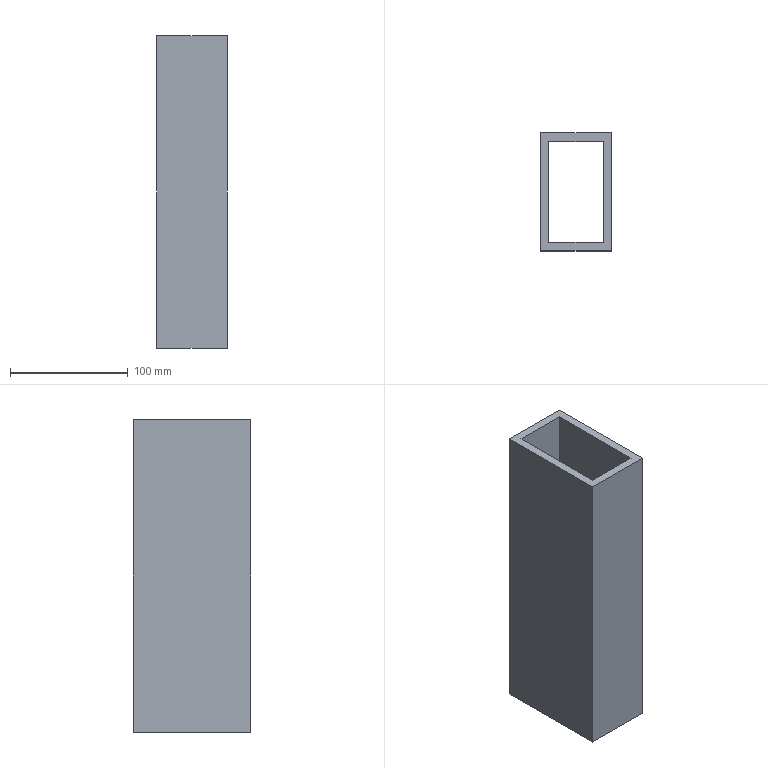Part | NX | features solid 2 | 1 solid | 10 faces | box 60 x 100 x 265 mm | volume 541660 mm3 | plane 10
STEP:
#1=CARTESIAN_POINT('',(-1138.,438.,210.));
#2=VERTEX_POINT('',#1);
#3=CARTESIAN_POINT('',(-1138.,352.,210.));
#4=VERTEX_POINT('',#3);
#5=CARTESIAN_POINT('',(-1138.,445.,210.));
#6=DIRECTION('',(0.,-1.,0.));
#7=VECTOR('',#6,1000.);
#8=LINE('',#5,#7);
#9=EDGE_CURVE('',#2,#4,#8,.T.);
#10=ORIENTED_EDGE('',*,*,#9,.T.);
#11=CARTESIAN_POINT('',(-1138.,352.,-55.));
#12=VERTEX_POINT('',#11);
#13=CARTESIAN_POINT('',(-1138.,352.,45.));
#14=DIRECTION('',(0.,0.,-1.));
#15=VECTOR('',#14,1000.);
#16=LINE('',#13,#15);
#17=EDGE_CURVE('',#4,#12,#16,.T.);
#18=ORIENTED_EDGE('',*,*,#17,.T.);
#19=CARTESIAN_POINT('',(-1138.,438.,-55.));
#20=VERTEX_POINT('',#19);
#21=CARTESIAN_POINT('',(-1138.,445.,-55.));
#22=DIRECTION('',(0.,-1.,0.));
#23=VECTOR('',#22,1000.);
#24=LINE('',#21,#23);
#25=EDGE_CURVE('',#20,#12,#24,.T.);
#26=ORIENTED_EDGE('',*,*,#25,.F.);
#27=CARTESIAN_POINT('',(-1138.,438.,45.));
#28=DIRECTION('',(0.,0.,1.));
#29=VECTOR('',#28,1000.);
#30=LINE('',#27,#29);
#31=EDGE_CURVE('',#20,#2,#30,.T.);
#32=ORIENTED_EDGE('',*,*,#31,.T.);
#33=EDGE_LOOP('',(#10,#18,#26,#32));
#34=FACE_BOUND('',#33,.T.);
#35=CARTESIAN_POINT('',(-1138.,495.,45.));
#36=DIRECTION('',(1.,0.,0.));
#37=DIRECTION('',(0.,0.,-1.));
#38=AXIS2_PLACEMENT_3D('',#35,#36,#37);
#39=PLANE('',#38);
#40=ADVANCED_FACE('',(#34),#39,.T.);
#41=CARTESIAN_POINT('',(-1092.,352.,210.));
#42=VERTEX_POINT('',#41);
#43=CARTESIAN_POINT('',(-1092.,352.,-55.));
#44=VERTEX_POINT('',#43);
#45=CARTESIAN_POINT('',(-1092.,352.,45.));
#46=DIRECTION('',(0.,0.,-1.));
#47=VECTOR('',#46,1000.);
#48=LINE('',#45,#47);
#49=EDGE_CURVE('',#42,#44,#48,.T.);
#50=ORIENTED_EDGE('',*,*,#49,.F.);
#51=CARTESIAN_POINT('',(-1092.,438.,210.));
#52=VERTEX_POINT('',#51);
#53=CARTESIAN_POINT('',(-1092.,445.,210.));
#54=DIRECTION('',(0.,-1.,0.));
#55=VECTOR('',#54,1000.);
#56=LINE('',#53,#55);
#57=EDGE_CURVE('',#52,#42,#56,.T.);
#58=ORIENTED_EDGE('',*,*,#57,.F.);
#59=CARTESIAN_POINT('',(-1092.,438.,-55.));
#60=VERTEX_POINT('',#59);
#61=CARTESIAN_POINT('',(-1092.,438.,45.));
#62=DIRECTION('',(0.,0.,1.));
#63=VECTOR('',#62,1000.);
#64=LINE('',#61,#63);
#65=EDGE_CURVE('',#60,#52,#64,.T.);
#66=ORIENTED_EDGE('',*,*,#65,.F.);
#67=CARTESIAN_POINT('',(-1092.,445.,-55.));
#68=DIRECTION('',(0.,-1.,0.));
#69=VECTOR('',#68,1000.);
#70=LINE('',#67,#69);
#71=EDGE_CURVE('',#60,#44,#70,.T.);
#72=ORIENTED_EDGE('',*,*,#71,.T.);
#73=EDGE_LOOP('',(#50,#58,#66,#72));
#74=FACE_BOUND('',#73,.T.);
#75=CARTESIAN_POINT('',(-1092.,495.,45.));
#76=DIRECTION('',(1.,0.,0.));
#77=DIRECTION('',(0.,0.,-1.));
#78=AXIS2_PLACEMENT_3D('',#75,#76,#77);
#79=PLANE('',#78);
#80=ADVANCED_FACE('',(#74),#79,.F.);
#81=CARTESIAN_POINT('',(-1145.,438.,-55.));
#82=DIRECTION('',(1.,0.,0.));
#83=VECTOR('',#82,1000.);
#84=LINE('',#81,#83);
#85=EDGE_CURVE('',#20,#60,#84,.T.);
#86=ORIENTED_EDGE('',*,*,#85,.T.);
#87=ORIENTED_EDGE('',*,*,#65,.T.);
#88=CARTESIAN_POINT('',(-1145.,438.,210.));
#89=DIRECTION('',(1.,0.,0.));
#90=VECTOR('',#89,1000.);
#91=LINE('',#88,#90);
#92=EDGE_CURVE('',#2,#52,#91,.T.);
#93=ORIENTED_EDGE('',*,*,#92,.F.);
#94=ORIENTED_EDGE('',*,*,#31,.F.);
#95=EDGE_LOOP('',(#86,#87,#93,#94));
#96=FACE_BOUND('',#95,.T.);
#97=CARTESIAN_POINT('',(-1145.,438.,45.));
#98=DIRECTION('',(0.,-1.,0.));
#99=DIRECTION('',(0.,0.,-1.));
#100=AXIS2_PLACEMENT_3D('',#97,#98,#99);
#101=PLANE('',#100);
#102=ADVANCED_FACE('',(#96),#101,.T.);
#103=ORIENTED_EDGE('',*,*,#57,.T.);
#104=CARTESIAN_POINT('',(-1145.,352.,210.));
#105=DIRECTION('',(1.,0.,0.));
#106=VECTOR('',#105,1000.);
#107=LINE('',#104,#106);
#108=EDGE_CURVE('',#4,#42,#107,.T.);
#109=ORIENTED_EDGE('',*,*,#108,.F.);
#110=ORIENTED_EDGE('',*,*,#9,.F.);
#111=ORIENTED_EDGE('',*,*,#92,.T.);
#112=EDGE_LOOP('',(#103,#109,#110,#111));
#113=FACE_BOUND('',#112,.T.);
#114=CARTESIAN_POINT('',(-1145.,345.,210.));
#115=VERTEX_POINT('',#114);
#116=CARTESIAN_POINT('',(-1085.,345.,210.));
#117=VERTEX_POINT('',#116);
#118=CARTESIAN_POINT('',(-1145.,345.,210.));
#119=DIRECTION('',(1.,0.,0.));
#120=VECTOR('',#119,1000.);
#121=LINE('',#118,#120);
#122=EDGE_CURVE('',#115,#117,#121,.T.);
#123=ORIENTED_EDGE('',*,*,#122,.T.);
#124=CARTESIAN_POINT('',(-1085.,445.,210.));
#125=VERTEX_POINT('',#124);
#126=CARTESIAN_POINT('',(-1085.,445.,210.));
#127=DIRECTION('',(0.,-1.,0.));
#128=VECTOR('',#127,1000.);
#129=LINE('',#126,#128);
#130=EDGE_CURVE('',#125,#117,#129,.T.);
#131=ORIENTED_EDGE('',*,*,#130,.F.);
#132=CARTESIAN_POINT('',(-1145.,445.,210.));
#133=VERTEX_POINT('',#132);
#134=CARTESIAN_POINT('',(-1145.,445.,210.));
#135=DIRECTION('',(1.,0.,0.));
#136=VECTOR('',#135,1000.);
#137=LINE('',#134,#136);
#138=EDGE_CURVE('',#133,#125,#137,.T.);
#139=ORIENTED_EDGE('',*,*,#138,.F.);
#140=CARTESIAN_POINT('',(-1145.,445.,210.));
#141=DIRECTION('',(0.,-1.,0.));
#142=VECTOR('',#141,1000.);
#143=LINE('',#140,#142);
#144=EDGE_CURVE('',#133,#115,#143,.T.);
#145=ORIENTED_EDGE('',*,*,#144,.T.);
#146=EDGE_LOOP('',(#123,#131,#139,#145));
#147=FACE_BOUND('',#146,.T.);
#148=CARTESIAN_POINT('',(-1145.,445.,210.));
#149=DIRECTION('',(0.,0.,-1.));
#150=DIRECTION('',(-1.,0.,0.));
#151=AXIS2_PLACEMENT_3D('',#148,#149,#150);
#152=PLANE('',#151);
#153=ADVANCED_FACE('',(#113,#147),#152,.F.);
#154=CARTESIAN_POINT('',(-1085.,345.,-55.));
#155=VERTEX_POINT('',#154);
#156=CARTESIAN_POINT('',(-1085.,345.,45.));
#157=DIRECTION('',(0.,0.,-1.));
#158=VECTOR('',#157,1000.);
#159=LINE('',#156,#158);
#160=EDGE_CURVE('',#117,#155,#159,.T.);
#161=ORIENTED_EDGE('',*,*,#160,.T.);
#162=CARTESIAN_POINT('',(-1085.,445.,-55.));
#163=VERTEX_POINT('',#162);
#164=CARTESIAN_POINT('',(-1085.,445.,-55.));
#165=DIRECTION('',(0.,-1.,0.));
#166=VECTOR('',#165,1000.);
#167=LINE('',#164,#166);
#168=EDGE_CURVE('',#163,#155,#167,.T.);
#169=ORIENTED_EDGE('',*,*,#168,.F.);
#170=CARTESIAN_POINT('',(-1085.,445.,45.));
#171=DIRECTION('',(0.,0.,-1.));
#172=VECTOR('',#171,1000.);
#173=LINE('',#170,#172);
#174=EDGE_CURVE('',#125,#163,#173,.T.);
#175=ORIENTED_EDGE('',*,*,#174,.F.);
#176=ORIENTED_EDGE('',*,*,#130,.T.);
#177=EDGE_LOOP('',(#161,#169,#175,#176));
#178=FACE_BOUND('',#177,.T.);
#179=CARTESIAN_POINT('',(-1085.,445.,45.));
#180=DIRECTION('',(-1.,0.,0.));
#181=DIRECTION('',(0.,0.,1.));
#182=AXIS2_PLACEMENT_3D('',#179,#180,#181);
#183=PLANE('',#182);
#184=ADVANCED_FACE('',(#178),#183,.F.);
#185=CARTESIAN_POINT('',(-1145.,352.,-55.));
#186=DIRECTION('',(1.,0.,0.));
#187=VECTOR('',#186,1000.);
#188=LINE('',#185,#187);
#189=EDGE_CURVE('',#12,#44,#188,.T.);
#190=ORIENTED_EDGE('',*,*,#189,.T.);
#191=ORIENTED_EDGE('',*,*,#71,.F.);
#192=ORIENTED_EDGE('',*,*,#85,.F.);
#193=ORIENTED_EDGE('',*,*,#25,.T.);
#194=EDGE_LOOP('',(#190,#191,#192,#193));
#195=FACE_BOUND('',#194,.T.);
#196=CARTESIAN_POINT('',(-1145.,345.,-55.));
#197=VERTEX_POINT('',#196);
#198=CARTESIAN_POINT('',(-1145.,345.,-55.));
#199=DIRECTION('',(1.,0.,0.));
#200=VECTOR('',#199,1000.);
#201=LINE('',#198,#200);
#202=EDGE_CURVE('',#197,#155,#201,.T.);
#203=ORIENTED_EDGE('',*,*,#202,.F.);
#204=CARTESIAN_POINT('',(-1145.,445.,-55.));
#205=VERTEX_POINT('',#204);
#206=CARTESIAN_POINT('',(-1145.,445.,-55.));
#207=DIRECTION('',(0.,-1.,0.));
#208=VECTOR('',#207,1000.);
#209=LINE('',#206,#208);
#210=EDGE_CURVE('',#205,#197,#209,.T.);
#211=ORIENTED_EDGE('',*,*,#210,.F.);
#212=CARTESIAN_POINT('',(-1145.,445.,-55.));
#213=DIRECTION('',(1.,0.,0.));
#214=VECTOR('',#213,1000.);
#215=LINE('',#212,#214);
#216=EDGE_CURVE('',#205,#163,#215,.T.);
#217=ORIENTED_EDGE('',*,*,#216,.T.);
#218=ORIENTED_EDGE('',*,*,#168,.T.);
#219=EDGE_LOOP('',(#203,#211,#217,#218));
#220=FACE_BOUND('',#219,.T.);
#221=CARTESIAN_POINT('',(-1145.,445.,-55.));
#222=DIRECTION('',(0.,0.,-1.));
#223=DIRECTION('',(-1.,0.,0.));
#224=AXIS2_PLACEMENT_3D('',#221,#222,#223);
#225=PLANE('',#224);
#226=ADVANCED_FACE('',(#195,#220),#225,.T.);
#227=CARTESIAN_POINT('',(-1145.,345.,45.));
#228=DIRECTION('',(0.,0.,-1.));
#229=VECTOR('',#228,1000.);
#230=LINE('',#227,#229);
#231=EDGE_CURVE('',#115,#197,#230,.T.);
#232=ORIENTED_EDGE('',*,*,#231,.F.);
#233=ORIENTED_EDGE('',*,*,#144,.F.);
#234=CARTESIAN_POINT('',(-1145.,445.,45.));
#235=DIRECTION('',(0.,0.,-1.));
#236=VECTOR('',#235,1000.);
#237=LINE('',#234,#236);
#238=EDGE_CURVE('',#133,#205,#237,.T.);
#239=ORIENTED_EDGE('',*,*,#238,.T.);
#240=ORIENTED_EDGE('',*,*,#210,.T.);
#241=EDGE_LOOP('',(#232,#233,#239,#240));
#242=FACE_BOUND('',#241,.T.);
#243=CARTESIAN_POINT('',(-1145.,445.,45.));
#244=DIRECTION('',(-1.,0.,0.));
#245=DIRECTION('',(0.,0.,1.));
#246=AXIS2_PLACEMENT_3D('',#243,#244,#245);
#247=PLANE('',#246);
#248=ADVANCED_FACE('',(#242),#247,.T.);
#249=ORIENTED_EDGE('',*,*,#174,.T.);
#250=ORIENTED_EDGE('',*,*,#216,.F.);
#251=ORIENTED_EDGE('',*,*,#238,.F.);
#252=ORIENTED_EDGE('',*,*,#138,.T.);
#253=EDGE_LOOP('',(#249,#250,#251,#252));
#254=FACE_BOUND('',#253,.T.);
#255=CARTESIAN_POINT('',(-1145.,445.,45.));
#256=DIRECTION('',(0.,-1.,0.));
#257=DIRECTION('',(0.,0.,-1.));
#258=AXIS2_PLACEMENT_3D('',#255,#256,#257);
#259=PLANE('',#258);
#260=ADVANCED_FACE('',(#254),#259,.F.);
#261=ORIENTED_EDGE('',*,*,#231,.T.);
#262=ORIENTED_EDGE('',*,*,#202,.T.);
#263=ORIENTED_EDGE('',*,*,#160,.F.);
#264=ORIENTED_EDGE('',*,*,#122,.F.);
#265=EDGE_LOOP('',(#261,#262,#263,#264));
#266=FACE_BOUND('',#265,.T.);
#267=CARTESIAN_POINT('',(-1145.,345.,45.));
#268=DIRECTION('',(0.,-1.,0.));
#269=DIRECTION('',(0.,0.,-1.));
#270=AXIS2_PLACEMENT_3D('',#267,#268,#269);
#271=PLANE('',#270);
#272=ADVANCED_FACE('',(#266),#271,.T.);
#273=ORIENTED_EDGE('',*,*,#17,.F.);
#274=ORIENTED_EDGE('',*,*,#108,.T.);
#275=ORIENTED_EDGE('',*,*,#49,.T.);
#276=ORIENTED_EDGE('',*,*,#189,.F.);
#277=EDGE_LOOP('',(#273,#274,#275,#276));
#278=FACE_BOUND('',#277,.T.);
#279=CARTESIAN_POINT('',(-1145.,352.,45.));
#280=DIRECTION('',(0.,-1.,0.));
#281=DIRECTION('',(0.,0.,-1.));
#282=AXIS2_PLACEMENT_3D('',#279,#280,#281);
#283=PLANE('',#282);
#284=ADVANCED_FACE('',(#278),#283,.F.);
#285=CLOSED_SHELL('',(#40,#80,#102,#153,#184,#226,#248,#260,#272,#284));
#286=MANIFOLD_SOLID_BREP('',#285);
#287=(LENGTH_UNIT()NAMED_UNIT(*)SI_UNIT(.MILLI.,.METRE.));
#288=UNCERTAINTY_MEASURE_WITH_UNIT(LENGTH_MEASURE(0.00001),#287,'','');
#289=(NAMED_UNIT(*)PLANE_ANGLE_UNIT()SI_UNIT($,.RADIAN.));
#290=(NAMED_UNIT(*)SI_UNIT($,.STERADIAN.)SOLID_ANGLE_UNIT());
#291=(GEOMETRIC_REPRESENTATION_CONTEXT(3)GLOBAL_UNCERTAINTY_ASSIGNED_CONTEXT((#288))GLOBAL_UNIT_ASSIGNED_CONTEXT((#287,#289,#290))REPRESENTATION_CONTEXT('',''));
#292=ADVANCED_BREP_SHAPE_REPRESENTATION('',(#286),#291);